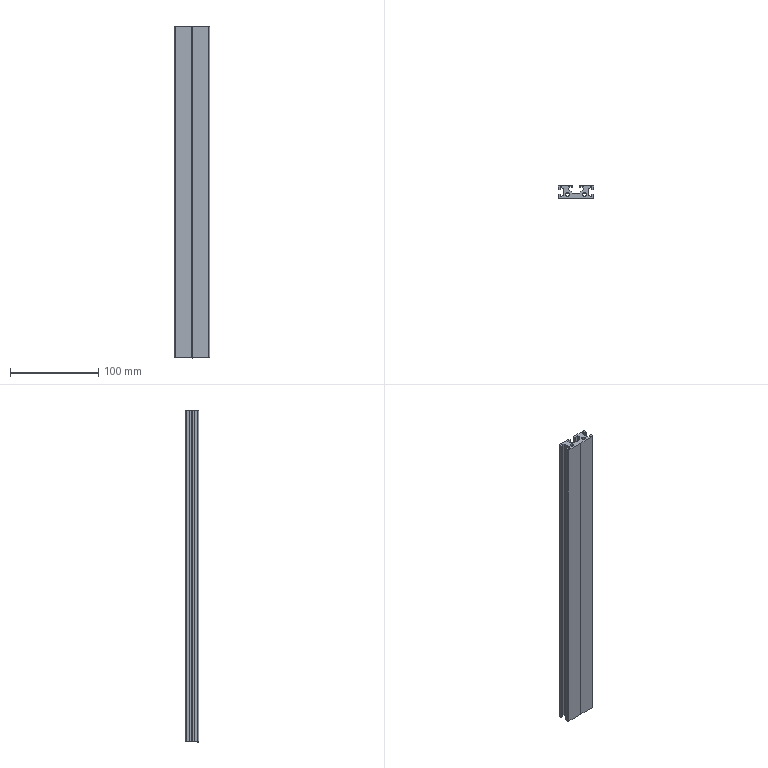Part | SolidWorks | features BaseBody 1, MoveFace 1 | 1 solid | 60 faces | box 40 x 15 x 377 mm | volume 132086 mm3 | plane 52 | cylinder 8 | commonest cylinder face diameters 2 x4 4.3 x4